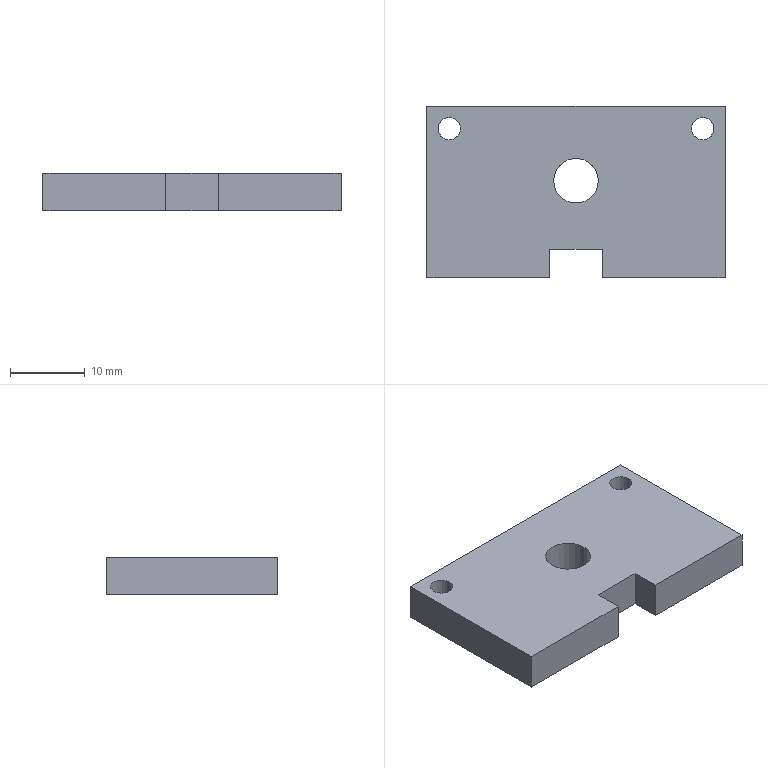Part | SolidWorks | features Extrusion 1 | 1 solid | 16 faces | box 40 x 23 x 5 mm | volume 4255 mm3 | plane 10 | cylinder 6 | commonest cylinder face diameters 3 x4 6 x2
STEP:
#1=CARTESIAN_POINT('',(15.5,7.,5.));
#2=VERTEX_POINT('',#1);
#3=CARTESIAN_POINT('',(18.5,7.,5.));
#4=VERTEX_POINT('',#3);
#5=CARTESIAN_POINT('',(17.,7.,5.));
#6=DIRECTION('',(0.,0.,1.));
#7=DIRECTION('',(1.,0.,0.));
#8=AXIS2_PLACEMENT_3D('',#5,#6,#7);
#9=CIRCLE('',#8,1.5);
#10=EDGE_CURVE('',#2,#4,#9,.T.);
#11=ORIENTED_EDGE('',*,*,#10,.T.);
#12=CARTESIAN_POINT('',(18.5,7.,0.));
#13=VERTEX_POINT('',#12);
#14=CARTESIAN_POINT('',(18.5,7.,5.));
#15=DIRECTION('',(0.,0.,-1.));
#16=VECTOR('',#15,1000.);
#17=LINE('',#14,#16);
#18=EDGE_CURVE('',#4,#13,#17,.T.);
#19=ORIENTED_EDGE('',*,*,#18,.T.);
#20=CARTESIAN_POINT('',(15.5,7.,0.));
#21=VERTEX_POINT('',#20);
#22=CARTESIAN_POINT('',(17.,7.,0.));
#23=DIRECTION('',(0.,0.,1.));
#24=DIRECTION('',(1.,0.,0.));
#25=AXIS2_PLACEMENT_3D('',#22,#23,#24);
#26=CIRCLE('',#25,1.5);
#27=EDGE_CURVE('',#21,#13,#26,.T.);
#28=ORIENTED_EDGE('',*,*,#27,.F.);
#29=CARTESIAN_POINT('',(15.5,7.,5.));
#30=DIRECTION('',(0.,0.,-1.));
#31=VECTOR('',#30,1000.);
#32=LINE('',#29,#31);
#33=EDGE_CURVE('',#2,#21,#32,.T.);
#34=ORIENTED_EDGE('',*,*,#33,.F.);
#35=EDGE_LOOP('',(#11,#19,#28,#34));
#36=FACE_OUTER_BOUND('',#35,.T.);
#37=CARTESIAN_POINT('',(17.,7.,5.));
#38=DIRECTION('',(0.,0.,-1.));
#39=DIRECTION('',(-1.,0.,0.));
#40=AXIS2_PLACEMENT_3D('',#37,#38,#39);
#41=CYLINDRICAL_SURFACE('',#40,1.5);
#42=ADVANCED_FACE('',(#36),#41,.F.);
#43=CARTESIAN_POINT('',(-18.5,7.,5.));
#44=VERTEX_POINT('',#43);
#45=CARTESIAN_POINT('',(-15.5,7.,5.));
#46=VERTEX_POINT('',#45);
#47=CARTESIAN_POINT('',(-17.,7.,5.));
#48=DIRECTION('',(0.,0.,1.));
#49=DIRECTION('',(1.,0.,0.));
#50=AXIS2_PLACEMENT_3D('',#47,#48,#49);
#51=CIRCLE('',#50,1.5);
#52=EDGE_CURVE('',#44,#46,#51,.T.);
#53=ORIENTED_EDGE('',*,*,#52,.T.);
#54=CARTESIAN_POINT('',(-15.5,7.,0.));
#55=VERTEX_POINT('',#54);
#56=CARTESIAN_POINT('',(-15.5,7.,5.));
#57=DIRECTION('',(0.,0.,-1.));
#58=VECTOR('',#57,1000.);
#59=LINE('',#56,#58);
#60=EDGE_CURVE('',#46,#55,#59,.T.);
#61=ORIENTED_EDGE('',*,*,#60,.T.);
#62=CARTESIAN_POINT('',(-18.5,7.,0.));
#63=VERTEX_POINT('',#62);
#64=CARTESIAN_POINT('',(-17.,7.,0.));
#65=DIRECTION('',(0.,0.,1.));
#66=DIRECTION('',(1.,0.,0.));
#67=AXIS2_PLACEMENT_3D('',#64,#65,#66);
#68=CIRCLE('',#67,1.5);
#69=EDGE_CURVE('',#63,#55,#68,.T.);
#70=ORIENTED_EDGE('',*,*,#69,.F.);
#71=CARTESIAN_POINT('',(-18.5,7.,5.));
#72=DIRECTION('',(0.,0.,-1.));
#73=VECTOR('',#72,1000.);
#74=LINE('',#71,#73);
#75=EDGE_CURVE('',#44,#63,#74,.T.);
#76=ORIENTED_EDGE('',*,*,#75,.F.);
#77=EDGE_LOOP('',(#53,#61,#70,#76));
#78=FACE_OUTER_BOUND('',#77,.T.);
#79=CARTESIAN_POINT('',(-17.,7.,5.));
#80=DIRECTION('',(0.,0.,-1.));
#81=DIRECTION('',(-1.,0.,0.));
#82=AXIS2_PLACEMENT_3D('',#79,#80,#81);
#83=CYLINDRICAL_SURFACE('',#82,1.5);
#84=ADVANCED_FACE('',(#78),#83,.F.);
#85=CARTESIAN_POINT('',(-3.,0.,5.));
#86=VERTEX_POINT('',#85);
#87=CARTESIAN_POINT('',(3.,0.,5.));
#88=VERTEX_POINT('',#87);
#89=CARTESIAN_POINT('',(0.,0.,5.));
#90=DIRECTION('',(0.,0.,1.));
#91=DIRECTION('',(1.,0.,0.));
#92=AXIS2_PLACEMENT_3D('',#89,#90,#91);
#93=CIRCLE('',#92,3.);
#94=EDGE_CURVE('',#86,#88,#93,.T.);
#95=ORIENTED_EDGE('',*,*,#94,.T.);
#96=CARTESIAN_POINT('',(3.,0.,0.));
#97=VERTEX_POINT('',#96);
#98=CARTESIAN_POINT('',(3.,0.,5.));
#99=DIRECTION('',(0.,0.,-1.));
#100=VECTOR('',#99,1000.);
#101=LINE('',#98,#100);
#102=EDGE_CURVE('',#88,#97,#101,.T.);
#103=ORIENTED_EDGE('',*,*,#102,.T.);
#104=CARTESIAN_POINT('',(-3.,0.,0.));
#105=VERTEX_POINT('',#104);
#106=CARTESIAN_POINT('',(0.,0.,0.));
#107=DIRECTION('',(0.,0.,1.));
#108=DIRECTION('',(1.,0.,0.));
#109=AXIS2_PLACEMENT_3D('',#106,#107,#108);
#110=CIRCLE('',#109,3.);
#111=EDGE_CURVE('',#105,#97,#110,.T.);
#112=ORIENTED_EDGE('',*,*,#111,.F.);
#113=CARTESIAN_POINT('',(-3.,0.,5.));
#114=DIRECTION('',(0.,0.,-1.));
#115=VECTOR('',#114,1000.);
#116=LINE('',#113,#115);
#117=EDGE_CURVE('',#86,#105,#116,.T.);
#118=ORIENTED_EDGE('',*,*,#117,.F.);
#119=EDGE_LOOP('',(#95,#103,#112,#118));
#120=FACE_OUTER_BOUND('',#119,.T.);
#121=CARTESIAN_POINT('',(0.,0.,5.));
#122=DIRECTION('',(0.,0.,-1.));
#123=DIRECTION('',(-1.,0.,0.));
#124=AXIS2_PLACEMENT_3D('',#121,#122,#123);
#125=CYLINDRICAL_SURFACE('',#124,3.);
#126=ADVANCED_FACE('',(#120),#125,.F.);
#127=CARTESIAN_POINT('',(20.,-13.,5.));
#128=VERTEX_POINT('',#127);
#129=CARTESIAN_POINT('',(20.,10.,5.));
#130=VERTEX_POINT('',#129);
#131=CARTESIAN_POINT('',(20.,-10.,5.));
#132=DIRECTION('',(0.,1.,0.));
#133=VECTOR('',#132,1000.);
#134=LINE('',#131,#133);
#135=EDGE_CURVE('',#128,#130,#134,.T.);
#136=ORIENTED_EDGE('',*,*,#135,.T.);
#137=CARTESIAN_POINT('',(-20.,10.,5.));
#138=VERTEX_POINT('',#137);
#139=CARTESIAN_POINT('',(-20.,10.,5.));
#140=DIRECTION('',(-1.,0.,0.));
#141=VECTOR('',#140,1000.);
#142=LINE('',#139,#141);
#143=EDGE_CURVE('',#130,#138,#142,.T.);
#144=ORIENTED_EDGE('',*,*,#143,.T.);
#145=CARTESIAN_POINT('',(-20.,-13.,5.));
#146=VERTEX_POINT('',#145);
#147=CARTESIAN_POINT('',(-20.,-10.,5.));
#148=DIRECTION('',(0.,-1.,0.));
#149=VECTOR('',#148,1000.);
#150=LINE('',#147,#149);
#151=EDGE_CURVE('',#138,#146,#150,.T.);
#152=ORIENTED_EDGE('',*,*,#151,.T.);
#153=CARTESIAN_POINT('',(-3.5,-13.,5.));
#154=VERTEX_POINT('',#153);
#155=CARTESIAN_POINT('',(-3.5,-13.,5.));
#156=DIRECTION('',(1.,0.,0.));
#157=VECTOR('',#156,1000.);
#158=LINE('',#155,#157);
#159=EDGE_CURVE('',#146,#154,#158,.T.);
#160=ORIENTED_EDGE('',*,*,#159,.T.);
#161=CARTESIAN_POINT('',(-3.5,-9.2,5.));
#162=VERTEX_POINT('',#161);
#163=CARTESIAN_POINT('',(-3.5,-9.2,5.));
#164=DIRECTION('',(0.,1.,0.));
#165=VECTOR('',#164,1000.);
#166=LINE('',#163,#165);
#167=EDGE_CURVE('',#154,#162,#166,.T.);
#168=ORIENTED_EDGE('',*,*,#167,.T.);
#169=CARTESIAN_POINT('',(3.5,-9.2,5.));
#170=VERTEX_POINT('',#169);
#171=CARTESIAN_POINT('',(3.5,-9.2,5.));
#172=DIRECTION('',(1.,0.,0.));
#173=VECTOR('',#172,1000.);
#174=LINE('',#171,#173);
#175=EDGE_CURVE('',#162,#170,#174,.T.);
#176=ORIENTED_EDGE('',*,*,#175,.T.);
#177=CARTESIAN_POINT('',(3.5,-13.,5.));
#178=VERTEX_POINT('',#177);
#179=CARTESIAN_POINT('',(3.5,-13.,5.));
#180=DIRECTION('',(0.,-1.,0.));
#181=VECTOR('',#180,1000.);
#182=LINE('',#179,#181);
#183=EDGE_CURVE('',#170,#178,#182,.T.);
#184=ORIENTED_EDGE('',*,*,#183,.T.);
#185=CARTESIAN_POINT('',(20.,-13.,5.));
#186=DIRECTION('',(1.,0.,0.));
#187=VECTOR('',#186,1000.);
#188=LINE('',#185,#187);
#189=EDGE_CURVE('',#178,#128,#188,.T.);
#190=ORIENTED_EDGE('',*,*,#189,.T.);
#191=EDGE_LOOP('',(#136,#144,#152,#160,#168,#176,#184,#190));
#192=FACE_OUTER_BOUND('',#191,.T.);
#193=ORIENTED_EDGE('',*,*,#94,.F.);
#194=CARTESIAN_POINT('',(0.,0.,5.));
#195=DIRECTION('',(0.,0.,1.));
#196=DIRECTION('',(1.,0.,0.));
#197=AXIS2_PLACEMENT_3D('',#194,#195,#196);
#198=CIRCLE('',#197,3.);
#199=EDGE_CURVE('',#88,#86,#198,.T.);
#200=ORIENTED_EDGE('',*,*,#199,.F.);
#201=EDGE_LOOP('',(#193,#200));
#202=FACE_BOUND('',#201,.T.);
#203=ORIENTED_EDGE('',*,*,#52,.F.);
#204=CARTESIAN_POINT('',(-17.,7.,5.));
#205=DIRECTION('',(0.,0.,1.));
#206=DIRECTION('',(1.,0.,0.));
#207=AXIS2_PLACEMENT_3D('',#204,#205,#206);
#208=CIRCLE('',#207,1.5);
#209=EDGE_CURVE('',#46,#44,#208,.T.);
#210=ORIENTED_EDGE('',*,*,#209,.F.);
#211=EDGE_LOOP('',(#203,#210));
#212=FACE_BOUND('',#211,.T.);
#213=ORIENTED_EDGE('',*,*,#10,.F.);
#214=CARTESIAN_POINT('',(17.,7.,5.));
#215=DIRECTION('',(0.,0.,1.));
#216=DIRECTION('',(1.,0.,0.));
#217=AXIS2_PLACEMENT_3D('',#214,#215,#216);
#218=CIRCLE('',#217,1.5);
#219=EDGE_CURVE('',#4,#2,#218,.T.);
#220=ORIENTED_EDGE('',*,*,#219,.F.);
#221=EDGE_LOOP('',(#213,#220));
#222=FACE_BOUND('',#221,.T.);
#223=CARTESIAN_POINT('',(0.,0.,5.));
#224=DIRECTION('',(0.,0.,-1.));
#225=DIRECTION('',(-1.,0.,0.));
#226=AXIS2_PLACEMENT_3D('',#223,#224,#225);
#227=PLANE('',#226);
#228=ADVANCED_FACE('',(#192,#202,#212,#222),#227,.F.);
#229=ORIENTED_EDGE('',*,*,#69,.T.);
#230=CARTESIAN_POINT('',(-17.,7.,0.));
#231=DIRECTION('',(0.,0.,1.));
#232=DIRECTION('',(1.,0.,0.));
#233=AXIS2_PLACEMENT_3D('',#230,#231,#232);
#234=CIRCLE('',#233,1.5);
#235=EDGE_CURVE('',#55,#63,#234,.T.);
#236=ORIENTED_EDGE('',*,*,#235,.T.);
#237=EDGE_LOOP('',(#229,#236));
#238=FACE_BOUND('',#237,.T.);
#239=CARTESIAN_POINT('',(20.,10.,0.));
#240=VERTEX_POINT('',#239);
#241=CARTESIAN_POINT('',(-20.,10.,0.));
#242=VERTEX_POINT('',#241);
#243=CARTESIAN_POINT('',(-20.,10.,0.));
#244=DIRECTION('',(-1.,0.,0.));
#245=VECTOR('',#244,1000.);
#246=LINE('',#243,#245);
#247=EDGE_CURVE('',#240,#242,#246,.T.);
#248=ORIENTED_EDGE('',*,*,#247,.F.);
#249=CARTESIAN_POINT('',(20.,-13.,0.));
#250=VERTEX_POINT('',#249);
#251=CARTESIAN_POINT('',(20.,-10.,0.));
#252=DIRECTION('',(0.,1.,0.));
#253=VECTOR('',#252,1000.);
#254=LINE('',#251,#253);
#255=EDGE_CURVE('',#250,#240,#254,.T.);
#256=ORIENTED_EDGE('',*,*,#255,.F.);
#257=CARTESIAN_POINT('',(3.5,-13.,0.));
#258=VERTEX_POINT('',#257);
#259=CARTESIAN_POINT('',(20.,-13.,0.));
#260=DIRECTION('',(1.,0.,0.));
#261=VECTOR('',#260,1000.);
#262=LINE('',#259,#261);
#263=EDGE_CURVE('',#258,#250,#262,.T.);
#264=ORIENTED_EDGE('',*,*,#263,.F.);
#265=CARTESIAN_POINT('',(3.5,-9.2,0.));
#266=VERTEX_POINT('',#265);
#267=CARTESIAN_POINT('',(3.5,-13.,0.));
#268=DIRECTION('',(0.,-1.,0.));
#269=VECTOR('',#268,1000.);
#270=LINE('',#267,#269);
#271=EDGE_CURVE('',#266,#258,#270,.T.);
#272=ORIENTED_EDGE('',*,*,#271,.F.);
#273=CARTESIAN_POINT('',(-3.5,-9.2,0.));
#274=VERTEX_POINT('',#273);
#275=CARTESIAN_POINT('',(3.5,-9.2,0.));
#276=DIRECTION('',(1.,0.,0.));
#277=VECTOR('',#276,1000.);
#278=LINE('',#275,#277);
#279=EDGE_CURVE('',#274,#266,#278,.T.);
#280=ORIENTED_EDGE('',*,*,#279,.F.);
#281=CARTESIAN_POINT('',(-3.5,-13.,0.));
#282=VERTEX_POINT('',#281);
#283=CARTESIAN_POINT('',(-3.5,-9.2,0.));
#284=DIRECTION('',(0.,1.,0.));
#285=VECTOR('',#284,1000.);
#286=LINE('',#283,#285);
#287=EDGE_CURVE('',#282,#274,#286,.T.);
#288=ORIENTED_EDGE('',*,*,#287,.F.);
#289=CARTESIAN_POINT('',(-20.,-13.,0.));
#290=VERTEX_POINT('',#289);
#291=CARTESIAN_POINT('',(-3.5,-13.,0.));
#292=DIRECTION('',(1.,0.,0.));
#293=VECTOR('',#292,1000.);
#294=LINE('',#291,#293);
#295=EDGE_CURVE('',#290,#282,#294,.T.);
#296=ORIENTED_EDGE('',*,*,#295,.F.);
#297=CARTESIAN_POINT('',(-20.,-10.,0.));
#298=DIRECTION('',(0.,-1.,0.));
#299=VECTOR('',#298,1000.);
#300=LINE('',#297,#299);
#301=EDGE_CURVE('',#242,#290,#300,.T.);
#302=ORIENTED_EDGE('',*,*,#301,.F.);
#303=EDGE_LOOP('',(#248,#256,#264,#272,#280,#288,#296,#302));
#304=FACE_OUTER_BOUND('',#303,.T.);
#305=ORIENTED_EDGE('',*,*,#111,.T.);
#306=CARTESIAN_POINT('',(0.,0.,0.));
#307=DIRECTION('',(0.,0.,1.));
#308=DIRECTION('',(1.,0.,0.));
#309=AXIS2_PLACEMENT_3D('',#306,#307,#308);
#310=CIRCLE('',#309,3.);
#311=EDGE_CURVE('',#97,#105,#310,.T.);
#312=ORIENTED_EDGE('',*,*,#311,.T.);
#313=EDGE_LOOP('',(#305,#312));
#314=FACE_BOUND('',#313,.T.);
#315=ORIENTED_EDGE('',*,*,#27,.T.);
#316=CARTESIAN_POINT('',(17.,7.,0.));
#317=DIRECTION('',(0.,0.,1.));
#318=DIRECTION('',(1.,0.,0.));
#319=AXIS2_PLACEMENT_3D('',#316,#317,#318);
#320=CIRCLE('',#319,1.5);
#321=EDGE_CURVE('',#13,#21,#320,.T.);
#322=ORIENTED_EDGE('',*,*,#321,.T.);
#323=EDGE_LOOP('',(#315,#322));
#324=FACE_BOUND('',#323,.T.);
#325=CARTESIAN_POINT('',(0.,0.,0.));
#326=DIRECTION('',(0.,0.,-1.));
#327=DIRECTION('',(-1.,0.,0.));
#328=AXIS2_PLACEMENT_3D('',#325,#326,#327);
#329=PLANE('',#328);
#330=ADVANCED_FACE('',(#238,#304,#314,#324),#329,.T.);
#331=ORIENTED_EDGE('',*,*,#247,.T.);
#332=CARTESIAN_POINT('',(-20.,10.,5.));
#333=DIRECTION('',(0.,0.,-1.));
#334=VECTOR('',#333,1000.);
#335=LINE('',#332,#334);
#336=EDGE_CURVE('',#138,#242,#335,.T.);
#337=ORIENTED_EDGE('',*,*,#336,.F.);
#338=ORIENTED_EDGE('',*,*,#143,.F.);
#339=CARTESIAN_POINT('',(20.,10.,5.));
#340=DIRECTION('',(0.,0.,-1.));
#341=VECTOR('',#340,1000.);
#342=LINE('',#339,#341);
#343=EDGE_CURVE('',#130,#240,#342,.T.);
#344=ORIENTED_EDGE('',*,*,#343,.T.);
#345=EDGE_LOOP('',(#331,#337,#338,#344));
#346=FACE_OUTER_BOUND('',#345,.T.);
#347=CARTESIAN_POINT('',(-20.,10.,5.));
#348=DIRECTION('',(0.,-1.,0.));
#349=DIRECTION('',(1.,0.,0.));
#350=AXIS2_PLACEMENT_3D('',#347,#348,#349);
#351=PLANE('',#350);
#352=ADVANCED_FACE('',(#346),#351,.F.);
#353=ORIENTED_EDGE('',*,*,#301,.T.);
#354=CARTESIAN_POINT('',(-20.,-13.,5.));
#355=DIRECTION('',(0.,0.,-1.));
#356=VECTOR('',#355,1000.);
#357=LINE('',#354,#356);
#358=EDGE_CURVE('',#146,#290,#357,.T.);
#359=ORIENTED_EDGE('',*,*,#358,.F.);
#360=ORIENTED_EDGE('',*,*,#151,.F.);
#361=ORIENTED_EDGE('',*,*,#336,.T.);
#362=EDGE_LOOP('',(#353,#359,#360,#361));
#363=FACE_OUTER_BOUND('',#362,.T.);
#364=CARTESIAN_POINT('',(-20.,-10.,5.));
#365=DIRECTION('',(1.,0.,0.));
#366=DIRECTION('',(0.,0.,-1.));
#367=AXIS2_PLACEMENT_3D('',#364,#365,#366);
#368=PLANE('',#367);
#369=ADVANCED_FACE('',(#363),#368,.F.);
#370=ORIENTED_EDGE('',*,*,#295,.T.);
#371=CARTESIAN_POINT('',(-3.5,-13.,5.));
#372=DIRECTION('',(0.,0.,-1.));
#373=VECTOR('',#372,1000.);
#374=LINE('',#371,#373);
#375=EDGE_CURVE('',#154,#282,#374,.T.);
#376=ORIENTED_EDGE('',*,*,#375,.F.);
#377=ORIENTED_EDGE('',*,*,#159,.F.);
#378=ORIENTED_EDGE('',*,*,#358,.T.);
#379=EDGE_LOOP('',(#370,#376,#377,#378));
#380=FACE_OUTER_BOUND('',#379,.T.);
#381=CARTESIAN_POINT('',(-3.5,-13.,5.));
#382=DIRECTION('',(0.,1.,0.));
#383=DIRECTION('',(-1.,0.,0.));
#384=AXIS2_PLACEMENT_3D('',#381,#382,#383);
#385=PLANE('',#384);
#386=ADVANCED_FACE('',(#380),#385,.F.);
#387=ORIENTED_EDGE('',*,*,#287,.T.);
#388=CARTESIAN_POINT('',(-3.5,-9.2,5.));
#389=DIRECTION('',(0.,0.,-1.));
#390=VECTOR('',#389,1000.);
#391=LINE('',#388,#390);
#392=EDGE_CURVE('',#162,#274,#391,.T.);
#393=ORIENTED_EDGE('',*,*,#392,.F.);
#394=ORIENTED_EDGE('',*,*,#167,.F.);
#395=ORIENTED_EDGE('',*,*,#375,.T.);
#396=EDGE_LOOP('',(#387,#393,#394,#395));
#397=FACE_OUTER_BOUND('',#396,.T.);
#398=CARTESIAN_POINT('',(-3.5,-9.2,5.));
#399=DIRECTION('',(-1.,0.,0.));
#400=DIRECTION('',(0.,-1.,0.));
#401=AXIS2_PLACEMENT_3D('',#398,#399,#400);
#402=PLANE('',#401);
#403=ADVANCED_FACE('',(#397),#402,.F.);
#404=ORIENTED_EDGE('',*,*,#279,.T.);
#405=CARTESIAN_POINT('',(3.5,-9.2,5.));
#406=DIRECTION('',(0.,0.,-1.));
#407=VECTOR('',#406,1000.);
#408=LINE('',#405,#407);
#409=EDGE_CURVE('',#170,#266,#408,.T.);
#410=ORIENTED_EDGE('',*,*,#409,.F.);
#411=ORIENTED_EDGE('',*,*,#175,.F.);
#412=ORIENTED_EDGE('',*,*,#392,.T.);
#413=EDGE_LOOP('',(#404,#410,#411,#412));
#414=FACE_OUTER_BOUND('',#413,.T.);
#415=CARTESIAN_POINT('',(3.5,-9.2,5.));
#416=DIRECTION('',(0.,1.,0.));
#417=DIRECTION('',(0.,0.,1.));
#418=AXIS2_PLACEMENT_3D('',#415,#416,#417);
#419=PLANE('',#418);
#420=ADVANCED_FACE('',(#414),#419,.F.);
#421=ORIENTED_EDGE('',*,*,#271,.T.);
#422=CARTESIAN_POINT('',(3.5,-13.,5.));
#423=DIRECTION('',(0.,0.,-1.));
#424=VECTOR('',#423,1000.);
#425=LINE('',#422,#424);
#426=EDGE_CURVE('',#178,#258,#425,.T.);
#427=ORIENTED_EDGE('',*,*,#426,.F.);
#428=ORIENTED_EDGE('',*,*,#183,.F.);
#429=ORIENTED_EDGE('',*,*,#409,.T.);
#430=EDGE_LOOP('',(#421,#427,#428,#429));
#431=FACE_OUTER_BOUND('',#430,.T.);
#432=CARTESIAN_POINT('',(3.5,-13.,5.));
#433=DIRECTION('',(1.,0.,0.));
#434=DIRECTION('',(0.,0.,-1.));
#435=AXIS2_PLACEMENT_3D('',#432,#433,#434);
#436=PLANE('',#435);
#437=ADVANCED_FACE('',(#431),#436,.F.);
#438=ORIENTED_EDGE('',*,*,#263,.T.);
#439=CARTESIAN_POINT('',(20.,-13.,5.));
#440=DIRECTION('',(0.,0.,-1.));
#441=VECTOR('',#440,1000.);
#442=LINE('',#439,#441);
#443=EDGE_CURVE('',#128,#250,#442,.T.);
#444=ORIENTED_EDGE('',*,*,#443,.F.);
#445=ORIENTED_EDGE('',*,*,#189,.F.);
#446=ORIENTED_EDGE('',*,*,#426,.T.);
#447=EDGE_LOOP('',(#438,#444,#445,#446));
#448=FACE_OUTER_BOUND('',#447,.T.);
#449=CARTESIAN_POINT('',(20.,-13.,5.));
#450=DIRECTION('',(0.,1.,0.));
#451=DIRECTION('',(0.,0.,1.));
#452=AXIS2_PLACEMENT_3D('',#449,#450,#451);
#453=PLANE('',#452);
#454=ADVANCED_FACE('',(#448),#453,.F.);
#455=ORIENTED_EDGE('',*,*,#255,.T.);
#456=ORIENTED_EDGE('',*,*,#343,.F.);
#457=ORIENTED_EDGE('',*,*,#135,.F.);
#458=ORIENTED_EDGE('',*,*,#443,.T.);
#459=EDGE_LOOP('',(#455,#456,#457,#458));
#460=FACE_OUTER_BOUND('',#459,.T.);
#461=CARTESIAN_POINT('',(20.,-10.,5.));
#462=DIRECTION('',(-1.,0.,0.));
#463=DIRECTION('',(0.,-1.,0.));
#464=AXIS2_PLACEMENT_3D('',#461,#462,#463);
#465=PLANE('',#464);
#466=ADVANCED_FACE('',(#460),#465,.F.);
#467=ORIENTED_EDGE('',*,*,#102,.F.);
#468=ORIENTED_EDGE('',*,*,#199,.T.);
#469=ORIENTED_EDGE('',*,*,#117,.T.);
#470=ORIENTED_EDGE('',*,*,#311,.F.);
#471=EDGE_LOOP('',(#467,#468,#469,#470));
#472=FACE_OUTER_BOUND('',#471,.T.);
#473=CARTESIAN_POINT('',(0.,0.,5.));
#474=DIRECTION('',(0.,0.,-1.));
#475=DIRECTION('',(-1.,0.,0.));
#476=AXIS2_PLACEMENT_3D('',#473,#474,#475);
#477=CYLINDRICAL_SURFACE('',#476,3.);
#478=ADVANCED_FACE('',(#472),#477,.F.);
#479=ORIENTED_EDGE('',*,*,#60,.F.);
#480=ORIENTED_EDGE('',*,*,#209,.T.);
#481=ORIENTED_EDGE('',*,*,#75,.T.);
#482=ORIENTED_EDGE('',*,*,#235,.F.);
#483=EDGE_LOOP('',(#479,#480,#481,#482));
#484=FACE_OUTER_BOUND('',#483,.T.);
#485=CARTESIAN_POINT('',(-17.,7.,5.));
#486=DIRECTION('',(0.,0.,-1.));
#487=DIRECTION('',(-1.,0.,0.));
#488=AXIS2_PLACEMENT_3D('',#485,#486,#487);
#489=CYLINDRICAL_SURFACE('',#488,1.5);
#490=ADVANCED_FACE('',(#484),#489,.F.);
#491=ORIENTED_EDGE('',*,*,#18,.F.);
#492=ORIENTED_EDGE('',*,*,#219,.T.);
#493=ORIENTED_EDGE('',*,*,#33,.T.);
#494=ORIENTED_EDGE('',*,*,#321,.F.);
#495=EDGE_LOOP('',(#491,#492,#493,#494));
#496=FACE_OUTER_BOUND('',#495,.T.);
#497=CARTESIAN_POINT('',(17.,7.,5.));
#498=DIRECTION('',(0.,0.,-1.));
#499=DIRECTION('',(-1.,0.,0.));
#500=AXIS2_PLACEMENT_3D('',#497,#498,#499);
#501=CYLINDRICAL_SURFACE('',#500,1.5);
#502=ADVANCED_FACE('',(#496),#501,.F.);
#503=CLOSED_SHELL('',(#42,#84,#126,#228,#330,#352,#369,#386,#403,#420,#437,#454,#466,#478,#490,#502));
#504=MANIFOLD_SOLID_BREP('',#503);
#505=CARTESIAN_POINT('',(0.,0.,0.));
#506=DIRECTION('',(0.,0.,1.));
#507=DIRECTION('',(1.,0.,0.));
#508=AXIS2_PLACEMENT_3D('',#505,#506,#507);
#509=(LENGTH_UNIT()NAMED_UNIT(*)SI_UNIT(.MILLI.,.METRE.));
#510=UNCERTAINTY_MEASURE_WITH_UNIT(LENGTH_MEASURE(0.00001),#509,'','');
#511=(NAMED_UNIT(*)PLANE_ANGLE_UNIT()SI_UNIT($,.RADIAN.));
#512=(NAMED_UNIT(*)SI_UNIT($,.STERADIAN.)SOLID_ANGLE_UNIT());
#513=(GEOMETRIC_REPRESENTATION_CONTEXT(3)GLOBAL_UNCERTAINTY_ASSIGNED_CONTEXT((#510))GLOBAL_UNIT_ASSIGNED_CONTEXT((#509,#511,#512))REPRESENTATION_CONTEXT('',''));
#514=ADVANCED_BREP_SHAPE_REPRESENTATION('',(#504,#508),#513);